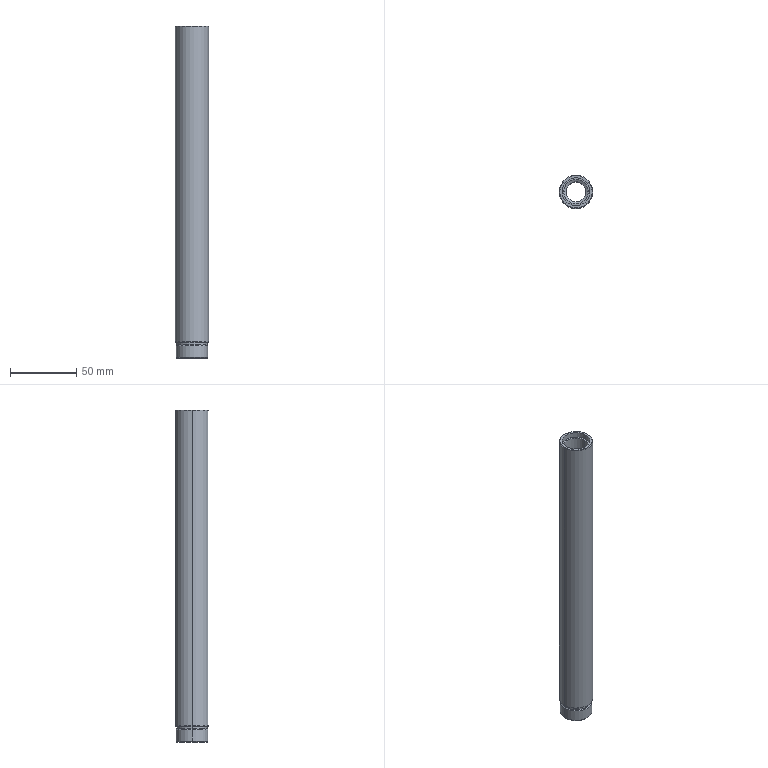Part | STEP file | 06活塞杆 EDA50-L_R-006-BZ^EDA50-R04 (D60N) | 1 solid | 28 faces | box 25 x 25 x 250 mm | volume 75291 mm3 | cone 12 | cylinder 12 | plane 4 | commonest cylinder face diameters 15 x2 18.5 x2 21 x2 22.8 x2 24 x2 25 x2